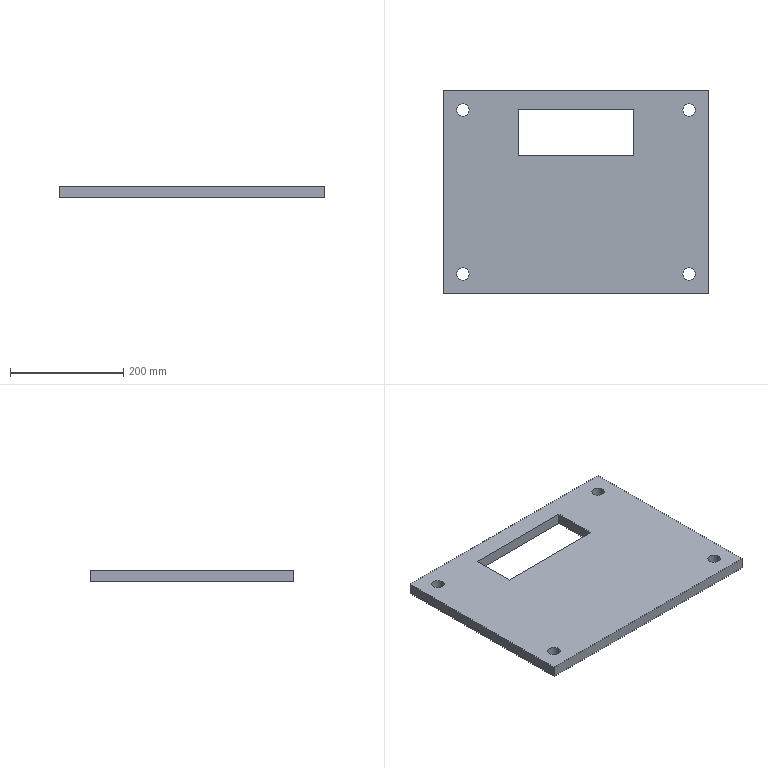Part | STEP file | Bearing seat fixing plate | 1 solid | 18 faces | box 470 x 360 x 20 mm | volume 3025589 mm3 | plane 10 | cylinder 8 | commonest cylinder face diameters 22 x8
STEP:
#1=CARTESIAN_POINT('',(0.,0.,0.));
#2=DIRECTION('',(0.,0.,1.));
#3=DIRECTION('',(1.,0.,0.));
#4=AXIS2_PLACEMENT_3D('',#1,#2,#3);
#5=CARTESIAN_POINT('',(424.,-325.,20.));
#6=VERTEX_POINT('',#5);
#7=CARTESIAN_POINT('',(424.,-325.,0.));
#8=VERTEX_POINT('',#7);
#9=CARTESIAN_POINT('',(424.,-325.,20.));
#10=DIRECTION('',(0.,0.,-1.));
#11=VECTOR('',#10,1.);
#12=LINE('',#9,#11);
#13=CARTESIAN_POINT('',(435.,-325.,20.));
#14=DIRECTION('',(0.,0.,-1.));
#15=DIRECTION('',(-1.,0.,0.));
#16=AXIS2_PLACEMENT_3D('',#13,#14,#15);
#17=CYLINDRICAL_SURFACE('',#16,11.);
#18=CARTESIAN_POINT('',(6.283,0.));
#19=DIRECTION('',(0.,1.));
#20=VECTOR('',#19,1.);
#21=LINE('',#18,#20);
#22=(GEOMETRIC_REPRESENTATION_CONTEXT(2)PARAMETRIC_REPRESENTATION_CONTEXT()REPRESENTATION_CONTEXT('',''));
#23=DEFINITIONAL_REPRESENTATION('',(#21),#22);
#24=PCURVE('',#17,#23);
#25=CARTESIAN_POINT('',(435.,-325.,20.));
#26=DIRECTION('',(0.,0.,-1.));
#27=DIRECTION('',(-1.,0.,0.));
#28=AXIS2_PLACEMENT_3D('',#25,#26,#27);
#29=CYLINDRICAL_SURFACE('',#28,11.);
#30=CARTESIAN_POINT('',(0.,0.));
#31=DIRECTION('',(0.,1.));
#32=VECTOR('',#31,1.);
#33=LINE('',#30,#32);
#34=(GEOMETRIC_REPRESENTATION_CONTEXT(2)PARAMETRIC_REPRESENTATION_CONTEXT()REPRESENTATION_CONTEXT('',''));
#35=DEFINITIONAL_REPRESENTATION('',(#33),#34);
#36=PCURVE('',#29,#35);
#37=SURFACE_CURVE('',#12,(#24,#36),.PCURVE_S1.);
#38=EDGE_CURVE('',#6,#8,#37,.T.);
#39=ORIENTED_EDGE('',*,*,#38,.T.);
#40=CARTESIAN_POINT('',(446.,-325.,0.));
#41=VERTEX_POINT('',#40);
#42=CARTESIAN_POINT('',(435.,-325.,0.));
#43=DIRECTION('',(0.,0.,1.));
#44=DIRECTION('',(1.,0.,0.));
#45=AXIS2_PLACEMENT_3D('',#42,#43,#44);
#46=CIRCLE('',#45,11.);
#47=CARTESIAN_POINT('',(9.425,20.));
#48=DIRECTION('',(-1.,0.));
#49=VECTOR('',#48,1.);
#50=LINE('',#47,#49);
#51=(GEOMETRIC_REPRESENTATION_CONTEXT(2)PARAMETRIC_REPRESENTATION_CONTEXT()REPRESENTATION_CONTEXT('',''));
#52=DEFINITIONAL_REPRESENTATION('',(#50),#51);
#53=PCURVE('',#17,#52);
#54=CARTESIAN_POINT('',(0.,0.,0.));
#55=DIRECTION('',(0.,0.,1.));
#56=DIRECTION('',(1.,0.,0.));
#57=AXIS2_PLACEMENT_3D('',#54,#55,#56);
#58=PLANE('',#57);
#59=CARTESIAN_POINT('',(435.,-325.));
#60=DIRECTION('',(1.,0.));
#61=AXIS2_PLACEMENT_2D('',#59,#60);
#62=CIRCLE('',#61,11.);
#63=(GEOMETRIC_REPRESENTATION_CONTEXT(2)PARAMETRIC_REPRESENTATION_CONTEXT()REPRESENTATION_CONTEXT('',''));
#64=DEFINITIONAL_REPRESENTATION('',(#62),#63);
#65=PCURVE('',#58,#64);
#66=SURFACE_CURVE('',#46,(#53,#65),.PCURVE_S1.);
#67=EDGE_CURVE('',#8,#41,#66,.T.);
#68=ORIENTED_EDGE('',*,*,#67,.T.);
#69=CARTESIAN_POINT('',(446.,-325.,20.));
#70=VERTEX_POINT('',#69);
#71=CARTESIAN_POINT('',(446.,-325.,20.));
#72=DIRECTION('',(0.,0.,-1.));
#73=VECTOR('',#72,1.);
#74=LINE('',#71,#73);
#75=CARTESIAN_POINT('',(3.142,0.));
#76=DIRECTION('',(0.,1.));
#77=VECTOR('',#76,1.);
#78=LINE('',#75,#77);
#79=(GEOMETRIC_REPRESENTATION_CONTEXT(2)PARAMETRIC_REPRESENTATION_CONTEXT()REPRESENTATION_CONTEXT('',''));
#80=DEFINITIONAL_REPRESENTATION('',(#78),#79);
#81=PCURVE('',#17,#80);
#82=CARTESIAN_POINT('',(3.142,0.));
#83=DIRECTION('',(0.,1.));
#84=VECTOR('',#83,1.);
#85=LINE('',#82,#84);
#86=(GEOMETRIC_REPRESENTATION_CONTEXT(2)PARAMETRIC_REPRESENTATION_CONTEXT()REPRESENTATION_CONTEXT('',''));
#87=DEFINITIONAL_REPRESENTATION('',(#85),#86);
#88=PCURVE('',#29,#87);
#89=SURFACE_CURVE('',#74,(#81,#88),.PCURVE_S1.);
#90=EDGE_CURVE('',#70,#41,#89,.T.);
#91=ORIENTED_EDGE('',*,*,#90,.F.);
#92=CARTESIAN_POINT('',(435.,-325.,20.));
#93=DIRECTION('',(0.,0.,1.));
#94=DIRECTION('',(1.,0.,0.));
#95=AXIS2_PLACEMENT_3D('',#92,#93,#94);
#96=CIRCLE('',#95,11.);
#97=CARTESIAN_POINT('',(9.425,0.));
#98=DIRECTION('',(-1.,0.));
#99=VECTOR('',#98,1.);
#100=LINE('',#97,#99);
#101=(GEOMETRIC_REPRESENTATION_CONTEXT(2)PARAMETRIC_REPRESENTATION_CONTEXT()REPRESENTATION_CONTEXT('',''));
#102=DEFINITIONAL_REPRESENTATION('',(#100),#101);
#103=PCURVE('',#17,#102);
#104=CARTESIAN_POINT('',(0.,0.,20.));
#105=DIRECTION('',(0.,0.,1.));
#106=DIRECTION('',(1.,0.,0.));
#107=AXIS2_PLACEMENT_3D('',#104,#105,#106);
#108=PLANE('',#107);
#109=CARTESIAN_POINT('',(435.,-325.));
#110=DIRECTION('',(1.,0.));
#111=AXIS2_PLACEMENT_2D('',#109,#110);
#112=CIRCLE('',#111,11.);
#113=(GEOMETRIC_REPRESENTATION_CONTEXT(2)PARAMETRIC_REPRESENTATION_CONTEXT()REPRESENTATION_CONTEXT('',''));
#114=DEFINITIONAL_REPRESENTATION('',(#112),#113);
#115=PCURVE('',#108,#114);
#116=SURFACE_CURVE('',#96,(#103,#115),.PCURVE_S1.);
#117=EDGE_CURVE('',#6,#70,#116,.T.);
#118=ORIENTED_EDGE('',*,*,#117,.F.);
#119=EDGE_LOOP('',(#39,#68,#91,#118));
#120=FACE_BOUND('',#119,.F.);
#121=ADVANCED_FACE('',(#120),#17,.F.);
#122=CARTESIAN_POINT('',(424.,-35.,20.));
#123=VERTEX_POINT('',#122);
#124=CARTESIAN_POINT('',(424.,-35.,0.));
#125=VERTEX_POINT('',#124);
#126=CARTESIAN_POINT('',(424.,-35.,20.));
#127=DIRECTION('',(0.,0.,-1.));
#128=VECTOR('',#127,1.);
#129=LINE('',#126,#128);
#130=CARTESIAN_POINT('',(435.,-35.,20.));
#131=DIRECTION('',(0.,0.,-1.));
#132=DIRECTION('',(-1.,0.,0.));
#133=AXIS2_PLACEMENT_3D('',#130,#131,#132);
#134=CYLINDRICAL_SURFACE('',#133,11.);
#135=CARTESIAN_POINT('',(6.283,0.));
#136=DIRECTION('',(0.,1.));
#137=VECTOR('',#136,1.);
#138=LINE('',#135,#137);
#139=(GEOMETRIC_REPRESENTATION_CONTEXT(2)PARAMETRIC_REPRESENTATION_CONTEXT()REPRESENTATION_CONTEXT('',''));
#140=DEFINITIONAL_REPRESENTATION('',(#138),#139);
#141=PCURVE('',#134,#140);
#142=CARTESIAN_POINT('',(435.,-35.,20.));
#143=DIRECTION('',(0.,0.,-1.));
#144=DIRECTION('',(-1.,0.,0.));
#145=AXIS2_PLACEMENT_3D('',#142,#143,#144);
#146=CYLINDRICAL_SURFACE('',#145,11.);
#147=CARTESIAN_POINT('',(0.,0.));
#148=DIRECTION('',(0.,1.));
#149=VECTOR('',#148,1.);
#150=LINE('',#147,#149);
#151=(GEOMETRIC_REPRESENTATION_CONTEXT(2)PARAMETRIC_REPRESENTATION_CONTEXT()REPRESENTATION_CONTEXT('',''));
#152=DEFINITIONAL_REPRESENTATION('',(#150),#151);
#153=PCURVE('',#146,#152);
#154=SURFACE_CURVE('',#129,(#141,#153),.PCURVE_S1.);
#155=EDGE_CURVE('',#123,#125,#154,.T.);
#156=ORIENTED_EDGE('',*,*,#155,.T.);
#157=CARTESIAN_POINT('',(446.,-35.,0.));
#158=VERTEX_POINT('',#157);
#159=CARTESIAN_POINT('',(435.,-35.,0.));
#160=DIRECTION('',(0.,0.,1.));
#161=DIRECTION('',(1.,0.,0.));
#162=AXIS2_PLACEMENT_3D('',#159,#160,#161);
#163=CIRCLE('',#162,11.);
#164=CARTESIAN_POINT('',(9.425,20.));
#165=DIRECTION('',(-1.,0.));
#166=VECTOR('',#165,1.);
#167=LINE('',#164,#166);
#168=(GEOMETRIC_REPRESENTATION_CONTEXT(2)PARAMETRIC_REPRESENTATION_CONTEXT()REPRESENTATION_CONTEXT('',''));
#169=DEFINITIONAL_REPRESENTATION('',(#167),#168);
#170=PCURVE('',#134,#169);
#171=CARTESIAN_POINT('',(435.,-35.));
#172=DIRECTION('',(1.,0.));
#173=AXIS2_PLACEMENT_2D('',#171,#172);
#174=CIRCLE('',#173,11.);
#175=(GEOMETRIC_REPRESENTATION_CONTEXT(2)PARAMETRIC_REPRESENTATION_CONTEXT()REPRESENTATION_CONTEXT('',''));
#176=DEFINITIONAL_REPRESENTATION('',(#174),#175);
#177=PCURVE('',#58,#176);
#178=SURFACE_CURVE('',#163,(#170,#177),.PCURVE_S1.);
#179=EDGE_CURVE('',#125,#158,#178,.T.);
#180=ORIENTED_EDGE('',*,*,#179,.T.);
#181=CARTESIAN_POINT('',(446.,-35.,20.));
#182=VERTEX_POINT('',#181);
#183=CARTESIAN_POINT('',(446.,-35.,20.));
#184=DIRECTION('',(0.,0.,-1.));
#185=VECTOR('',#184,1.);
#186=LINE('',#183,#185);
#187=CARTESIAN_POINT('',(3.142,0.));
#188=DIRECTION('',(0.,1.));
#189=VECTOR('',#188,1.);
#190=LINE('',#187,#189);
#191=(GEOMETRIC_REPRESENTATION_CONTEXT(2)PARAMETRIC_REPRESENTATION_CONTEXT()REPRESENTATION_CONTEXT('',''));
#192=DEFINITIONAL_REPRESENTATION('',(#190),#191);
#193=PCURVE('',#134,#192);
#194=CARTESIAN_POINT('',(3.142,0.));
#195=DIRECTION('',(0.,1.));
#196=VECTOR('',#195,1.);
#197=LINE('',#194,#196);
#198=(GEOMETRIC_REPRESENTATION_CONTEXT(2)PARAMETRIC_REPRESENTATION_CONTEXT()REPRESENTATION_CONTEXT('',''));
#199=DEFINITIONAL_REPRESENTATION('',(#197),#198);
#200=PCURVE('',#146,#199);
#201=SURFACE_CURVE('',#186,(#193,#200),.PCURVE_S1.);
#202=EDGE_CURVE('',#182,#158,#201,.T.);
#203=ORIENTED_EDGE('',*,*,#202,.F.);
#204=CARTESIAN_POINT('',(435.,-35.,20.));
#205=DIRECTION('',(0.,0.,1.));
#206=DIRECTION('',(1.,0.,0.));
#207=AXIS2_PLACEMENT_3D('',#204,#205,#206);
#208=CIRCLE('',#207,11.);
#209=CARTESIAN_POINT('',(9.425,0.));
#210=DIRECTION('',(-1.,0.));
#211=VECTOR('',#210,1.);
#212=LINE('',#209,#211);
#213=(GEOMETRIC_REPRESENTATION_CONTEXT(2)PARAMETRIC_REPRESENTATION_CONTEXT()REPRESENTATION_CONTEXT('',''));
#214=DEFINITIONAL_REPRESENTATION('',(#212),#213);
#215=PCURVE('',#134,#214);
#216=CARTESIAN_POINT('',(435.,-35.));
#217=DIRECTION('',(1.,0.));
#218=AXIS2_PLACEMENT_2D('',#216,#217);
#219=CIRCLE('',#218,11.);
#220=(GEOMETRIC_REPRESENTATION_CONTEXT(2)PARAMETRIC_REPRESENTATION_CONTEXT()REPRESENTATION_CONTEXT('',''));
#221=DEFINITIONAL_REPRESENTATION('',(#219),#220);
#222=PCURVE('',#108,#221);
#223=SURFACE_CURVE('',#208,(#215,#222),.PCURVE_S1.);
#224=EDGE_CURVE('',#123,#182,#223,.T.);
#225=ORIENTED_EDGE('',*,*,#224,.F.);
#226=EDGE_LOOP('',(#156,#180,#203,#225));
#227=FACE_BOUND('',#226,.F.);
#228=ADVANCED_FACE('',(#227),#134,.F.);
#229=CARTESIAN_POINT('',(24.,-325.,20.));
#230=VERTEX_POINT('',#229);
#231=CARTESIAN_POINT('',(24.,-325.,0.));
#232=VERTEX_POINT('',#231);
#233=CARTESIAN_POINT('',(24.,-325.,20.));
#234=DIRECTION('',(0.,0.,-1.));
#235=VECTOR('',#234,1.);
#236=LINE('',#233,#235);
#237=CARTESIAN_POINT('',(35.,-325.,20.));
#238=DIRECTION('',(0.,0.,-1.));
#239=DIRECTION('',(-1.,0.,0.));
#240=AXIS2_PLACEMENT_3D('',#237,#238,#239);
#241=CYLINDRICAL_SURFACE('',#240,11.);
#242=CARTESIAN_POINT('',(6.283,0.));
#243=DIRECTION('',(0.,1.));
#244=VECTOR('',#243,1.);
#245=LINE('',#242,#244);
#246=(GEOMETRIC_REPRESENTATION_CONTEXT(2)PARAMETRIC_REPRESENTATION_CONTEXT()REPRESENTATION_CONTEXT('',''));
#247=DEFINITIONAL_REPRESENTATION('',(#245),#246);
#248=PCURVE('',#241,#247);
#249=CARTESIAN_POINT('',(35.,-325.,20.));
#250=DIRECTION('',(0.,0.,-1.));
#251=DIRECTION('',(-1.,0.,0.));
#252=AXIS2_PLACEMENT_3D('',#249,#250,#251);
#253=CYLINDRICAL_SURFACE('',#252,11.);
#254=CARTESIAN_POINT('',(0.,0.));
#255=DIRECTION('',(0.,1.));
#256=VECTOR('',#255,1.);
#257=LINE('',#254,#256);
#258=(GEOMETRIC_REPRESENTATION_CONTEXT(2)PARAMETRIC_REPRESENTATION_CONTEXT()REPRESENTATION_CONTEXT('',''));
#259=DEFINITIONAL_REPRESENTATION('',(#257),#258);
#260=PCURVE('',#253,#259);
#261=SURFACE_CURVE('',#236,(#248,#260),.PCURVE_S1.);
#262=EDGE_CURVE('',#230,#232,#261,.T.);
#263=ORIENTED_EDGE('',*,*,#262,.T.);
#264=CARTESIAN_POINT('',(46.,-325.,0.));
#265=VERTEX_POINT('',#264);
#266=CARTESIAN_POINT('',(35.,-325.,0.));
#267=DIRECTION('',(0.,0.,1.));
#268=DIRECTION('',(1.,0.,0.));
#269=AXIS2_PLACEMENT_3D('',#266,#267,#268);
#270=CIRCLE('',#269,11.);
#271=CARTESIAN_POINT('',(9.425,20.));
#272=DIRECTION('',(-1.,0.));
#273=VECTOR('',#272,1.);
#274=LINE('',#271,#273);
#275=(GEOMETRIC_REPRESENTATION_CONTEXT(2)PARAMETRIC_REPRESENTATION_CONTEXT()REPRESENTATION_CONTEXT('',''));
#276=DEFINITIONAL_REPRESENTATION('',(#274),#275);
#277=PCURVE('',#241,#276);
#278=CARTESIAN_POINT('',(35.,-325.));
#279=DIRECTION('',(1.,0.));
#280=AXIS2_PLACEMENT_2D('',#278,#279);
#281=CIRCLE('',#280,11.);
#282=(GEOMETRIC_REPRESENTATION_CONTEXT(2)PARAMETRIC_REPRESENTATION_CONTEXT()REPRESENTATION_CONTEXT('',''));
#283=DEFINITIONAL_REPRESENTATION('',(#281),#282);
#284=PCURVE('',#58,#283);
#285=SURFACE_CURVE('',#270,(#277,#284),.PCURVE_S1.);
#286=EDGE_CURVE('',#232,#265,#285,.T.);
#287=ORIENTED_EDGE('',*,*,#286,.T.);
#288=CARTESIAN_POINT('',(46.,-325.,20.));
#289=VERTEX_POINT('',#288);
#290=CARTESIAN_POINT('',(46.,-325.,20.));
#291=DIRECTION('',(0.,0.,-1.));
#292=VECTOR('',#291,1.);
#293=LINE('',#290,#292);
#294=CARTESIAN_POINT('',(3.142,0.));
#295=DIRECTION('',(0.,1.));
#296=VECTOR('',#295,1.);
#297=LINE('',#294,#296);
#298=(GEOMETRIC_REPRESENTATION_CONTEXT(2)PARAMETRIC_REPRESENTATION_CONTEXT()REPRESENTATION_CONTEXT('',''));
#299=DEFINITIONAL_REPRESENTATION('',(#297),#298);
#300=PCURVE('',#241,#299);
#301=CARTESIAN_POINT('',(3.142,0.));
#302=DIRECTION('',(0.,1.));
#303=VECTOR('',#302,1.);
#304=LINE('',#301,#303);
#305=(GEOMETRIC_REPRESENTATION_CONTEXT(2)PARAMETRIC_REPRESENTATION_CONTEXT()REPRESENTATION_CONTEXT('',''));
#306=DEFINITIONAL_REPRESENTATION('',(#304),#305);
#307=PCURVE('',#253,#306);
#308=SURFACE_CURVE('',#293,(#300,#307),.PCURVE_S1.);
#309=EDGE_CURVE('',#289,#265,#308,.T.);
#310=ORIENTED_EDGE('',*,*,#309,.F.);
#311=CARTESIAN_POINT('',(35.,-325.,20.));
#312=DIRECTION('',(0.,0.,1.));
#313=DIRECTION('',(1.,0.,0.));
#314=AXIS2_PLACEMENT_3D('',#311,#312,#313);
#315=CIRCLE('',#314,11.);
#316=CARTESIAN_POINT('',(9.425,0.));
#317=DIRECTION('',(-1.,0.));
#318=VECTOR('',#317,1.);
#319=LINE('',#316,#318);
#320=(GEOMETRIC_REPRESENTATION_CONTEXT(2)PARAMETRIC_REPRESENTATION_CONTEXT()REPRESENTATION_CONTEXT('',''));
#321=DEFINITIONAL_REPRESENTATION('',(#319),#320);
#322=PCURVE('',#241,#321);
#323=CARTESIAN_POINT('',(35.,-325.));
#324=DIRECTION('',(1.,0.));
#325=AXIS2_PLACEMENT_2D('',#323,#324);
#326=CIRCLE('',#325,11.);
#327=(GEOMETRIC_REPRESENTATION_CONTEXT(2)PARAMETRIC_REPRESENTATION_CONTEXT()REPRESENTATION_CONTEXT('',''));
#328=DEFINITIONAL_REPRESENTATION('',(#326),#327);
#329=PCURVE('',#108,#328);
#330=SURFACE_CURVE('',#315,(#322,#329),.PCURVE_S1.);
#331=EDGE_CURVE('',#230,#289,#330,.T.);
#332=ORIENTED_EDGE('',*,*,#331,.F.);
#333=EDGE_LOOP('',(#263,#287,#310,#332));
#334=FACE_BOUND('',#333,.F.);
#335=ADVANCED_FACE('',(#334),#241,.F.);
#336=CARTESIAN_POINT('',(24.,-35.,20.));
#337=VERTEX_POINT('',#336);
#338=CARTESIAN_POINT('',(24.,-35.,0.));
#339=VERTEX_POINT('',#338);
#340=CARTESIAN_POINT('',(24.,-35.,20.));
#341=DIRECTION('',(0.,0.,-1.));
#342=VECTOR('',#341,1.);
#343=LINE('',#340,#342);
#344=CARTESIAN_POINT('',(35.,-35.,20.));
#345=DIRECTION('',(0.,0.,-1.));
#346=DIRECTION('',(-1.,0.,0.));
#347=AXIS2_PLACEMENT_3D('',#344,#345,#346);
#348=CYLINDRICAL_SURFACE('',#347,11.);
#349=CARTESIAN_POINT('',(6.283,0.));
#350=DIRECTION('',(0.,1.));
#351=VECTOR('',#350,1.);
#352=LINE('',#349,#351);
#353=(GEOMETRIC_REPRESENTATION_CONTEXT(2)PARAMETRIC_REPRESENTATION_CONTEXT()REPRESENTATION_CONTEXT('',''));
#354=DEFINITIONAL_REPRESENTATION('',(#352),#353);
#355=PCURVE('',#348,#354);
#356=CARTESIAN_POINT('',(35.,-35.,20.));
#357=DIRECTION('',(0.,0.,-1.));
#358=DIRECTION('',(-1.,0.,0.));
#359=AXIS2_PLACEMENT_3D('',#356,#357,#358);
#360=CYLINDRICAL_SURFACE('',#359,11.);
#361=CARTESIAN_POINT('',(0.,0.));
#362=DIRECTION('',(0.,1.));
#363=VECTOR('',#362,1.);
#364=LINE('',#361,#363);
#365=(GEOMETRIC_REPRESENTATION_CONTEXT(2)PARAMETRIC_REPRESENTATION_CONTEXT()REPRESENTATION_CONTEXT('',''));
#366=DEFINITIONAL_REPRESENTATION('',(#364),#365);
#367=PCURVE('',#360,#366);
#368=SURFACE_CURVE('',#343,(#355,#367),.PCURVE_S1.);
#369=EDGE_CURVE('',#337,#339,#368,.T.);
#370=ORIENTED_EDGE('',*,*,#369,.T.);
#371=CARTESIAN_POINT('',(46.,-35.,0.));
#372=VERTEX_POINT('',#371);
#373=CARTESIAN_POINT('',(35.,-35.,0.));
#374=DIRECTION('',(0.,0.,1.));
#375=DIRECTION('',(1.,0.,0.));
#376=AXIS2_PLACEMENT_3D('',#373,#374,#375);
#377=CIRCLE('',#376,11.);
#378=CARTESIAN_POINT('',(9.425,20.));
#379=DIRECTION('',(-1.,0.));
#380=VECTOR('',#379,1.);
#381=LINE('',#378,#380);
#382=(GEOMETRIC_REPRESENTATION_CONTEXT(2)PARAMETRIC_REPRESENTATION_CONTEXT()REPRESENTATION_CONTEXT('',''));
#383=DEFINITIONAL_REPRESENTATION('',(#381),#382);
#384=PCURVE('',#348,#383);
#385=CARTESIAN_POINT('',(35.,-35.));
#386=DIRECTION('',(1.,0.));
#387=AXIS2_PLACEMENT_2D('',#385,#386);
#388=CIRCLE('',#387,11.);
#389=(GEOMETRIC_REPRESENTATION_CONTEXT(2)PARAMETRIC_REPRESENTATION_CONTEXT()REPRESENTATION_CONTEXT('',''));
#390=DEFINITIONAL_REPRESENTATION('',(#388),#389);
#391=PCURVE('',#58,#390);
#392=SURFACE_CURVE('',#377,(#384,#391),.PCURVE_S1.);
#393=EDGE_CURVE('',#339,#372,#392,.T.);
#394=ORIENTED_EDGE('',*,*,#393,.T.);
#395=CARTESIAN_POINT('',(46.,-35.,20.));
#396=VERTEX_POINT('',#395);
#397=CARTESIAN_POINT('',(46.,-35.,20.));
#398=DIRECTION('',(0.,0.,-1.));
#399=VECTOR('',#398,1.);
#400=LINE('',#397,#399);
#401=CARTESIAN_POINT('',(3.142,0.));
#402=DIRECTION('',(0.,1.));
#403=VECTOR('',#402,1.);
#404=LINE('',#401,#403);
#405=(GEOMETRIC_REPRESENTATION_CONTEXT(2)PARAMETRIC_REPRESENTATION_CONTEXT()REPRESENTATION_CONTEXT('',''));
#406=DEFINITIONAL_REPRESENTATION('',(#404),#405);
#407=PCURVE('',#348,#406);
#408=CARTESIAN_POINT('',(3.142,0.));
#409=DIRECTION('',(0.,1.));
#410=VECTOR('',#409,1.);
#411=LINE('',#408,#410);
#412=(GEOMETRIC_REPRESENTATION_CONTEXT(2)PARAMETRIC_REPRESENTATION_CONTEXT()REPRESENTATION_CONTEXT('',''));
#413=DEFINITIONAL_REPRESENTATION('',(#411),#412);
#414=PCURVE('',#360,#413);
#415=SURFACE_CURVE('',#400,(#407,#414),.PCURVE_S1.);
#416=EDGE_CURVE('',#396,#372,#415,.T.);
#417=ORIENTED_EDGE('',*,*,#416,.F.);
#418=CARTESIAN_POINT('',(35.,-35.,20.));
#419=DIRECTION('',(0.,0.,1.));
#420=DIRECTION('',(1.,0.,0.));
#421=AXIS2_PLACEMENT_3D('',#418,#419,#420);
#422=CIRCLE('',#421,11.);
#423=CARTESIAN_POINT('',(9.425,0.));
#424=DIRECTION('',(-1.,0.));
#425=VECTOR('',#424,1.);
#426=LINE('',#423,#425);
#427=(GEOMETRIC_REPRESENTATION_CONTEXT(2)PARAMETRIC_REPRESENTATION_CONTEXT()REPRESENTATION_CONTEXT('',''));
#428=DEFINITIONAL_REPRESENTATION('',(#426),#427);
#429=PCURVE('',#348,#428);
#430=CARTESIAN_POINT('',(35.,-35.));
#431=DIRECTION('',(1.,0.));
#432=AXIS2_PLACEMENT_2D('',#430,#431);
#433=CIRCLE('',#432,11.);
#434=(GEOMETRIC_REPRESENTATION_CONTEXT(2)PARAMETRIC_REPRESENTATION_CONTEXT()REPRESENTATION_CONTEXT('',''));
#435=DEFINITIONAL_REPRESENTATION('',(#433),#434);
#436=PCURVE('',#108,#435);
#437=SURFACE_CURVE('',#422,(#429,#436),.PCURVE_S1.);
#438=EDGE_CURVE('',#337,#396,#437,.T.);
#439=ORIENTED_EDGE('',*,*,#438,.F.);
#440=EDGE_LOOP('',(#370,#394,#417,#439));
#441=FACE_BOUND('',#440,.F.);
#442=ADVANCED_FACE('',(#441),#348,.F.);
#443=ORIENTED_EDGE('',*,*,#224,.F.);
#444=CARTESIAN_POINT('',(435.,-35.,20.));
#445=DIRECTION('',(0.,0.,1.));
#446=DIRECTION('',(1.,0.,0.));
#447=AXIS2_PLACEMENT_3D('',#444,#445,#446);
#448=CIRCLE('',#447,11.);
#449=CARTESIAN_POINT('',(435.,-35.));
#450=DIRECTION('',(1.,0.));
#451=AXIS2_PLACEMENT_2D('',#449,#450);
#452=CIRCLE('',#451,11.);
#453=(GEOMETRIC_REPRESENTATION_CONTEXT(2)PARAMETRIC_REPRESENTATION_CONTEXT()REPRESENTATION_CONTEXT('',''));
#454=DEFINITIONAL_REPRESENTATION('',(#452),#453);
#455=PCURVE('',#108,#454);
#456=CARTESIAN_POINT('',(3.142,0.));
#457=DIRECTION('',(-1.,0.));
#458=VECTOR('',#457,1.);
#459=LINE('',#456,#458);
#460=(GEOMETRIC_REPRESENTATION_CONTEXT(2)PARAMETRIC_REPRESENTATION_CONTEXT()REPRESENTATION_CONTEXT('',''));
#461=DEFINITIONAL_REPRESENTATION('',(#459),#460);
#462=PCURVE('',#146,#461);
#463=SURFACE_CURVE('',#448,(#455,#462),.PCURVE_S1.);
#464=EDGE_CURVE('',#182,#123,#463,.T.);
#465=ORIENTED_EDGE('',*,*,#464,.F.);
#466=EDGE_LOOP('',(#443,#465));
#467=FACE_BOUND('',#466,.T.);
#468=ORIENTED_EDGE('',*,*,#438,.F.);
#469=CARTESIAN_POINT('',(35.,-35.,20.));
#470=DIRECTION('',(0.,0.,1.));
#471=DIRECTION('',(1.,0.,0.));
#472=AXIS2_PLACEMENT_3D('',#469,#470,#471);
#473=CIRCLE('',#472,11.);
#474=CARTESIAN_POINT('',(35.,-35.));
#475=DIRECTION('',(1.,0.));
#476=AXIS2_PLACEMENT_2D('',#474,#475);
#477=CIRCLE('',#476,11.);
#478=(GEOMETRIC_REPRESENTATION_CONTEXT(2)PARAMETRIC_REPRESENTATION_CONTEXT()REPRESENTATION_CONTEXT('',''));
#479=DEFINITIONAL_REPRESENTATION('',(#477),#478);
#480=PCURVE('',#108,#479);
#481=CARTESIAN_POINT('',(3.142,0.));
#482=DIRECTION('',(-1.,0.));
#483=VECTOR('',#482,1.);
#484=LINE('',#481,#483);
#485=(GEOMETRIC_REPRESENTATION_CONTEXT(2)PARAMETRIC_REPRESENTATION_CONTEXT()REPRESENTATION_CONTEXT('',''));
#486=DEFINITIONAL_REPRESENTATION('',(#484),#485);
#487=PCURVE('',#360,#486);
#488=SURFACE_CURVE('',#473,(#480,#487),.PCURVE_S1.);
#489=EDGE_CURVE('',#396,#337,#488,.T.);
#490=ORIENTED_EDGE('',*,*,#489,.F.);
#491=EDGE_LOOP('',(#468,#490));
#492=FACE_BOUND('',#491,.T.);
#493=CARTESIAN_POINT('',(0.,0.,20.));
#494=VERTEX_POINT('',#493);
#495=CARTESIAN_POINT('',(0.,-360.,20.));
#496=VERTEX_POINT('',#495);
#497=CARTESIAN_POINT('',(0.,0.,20.));
#498=DIRECTION('',(0.,-1.,0.));
#499=VECTOR('',#498,1.);
#500=LINE('',#497,#499);
#501=CARTESIAN_POINT('',(0.,0.));
#502=DIRECTION('',(0.,-1.));
#503=VECTOR('',#502,1.);
#504=LINE('',#501,#503);
#505=(GEOMETRIC_REPRESENTATION_CONTEXT(2)PARAMETRIC_REPRESENTATION_CONTEXT()REPRESENTATION_CONTEXT('',''));
#506=DEFINITIONAL_REPRESENTATION('',(#504),#505);
#507=PCURVE('',#108,#506);
#508=CARTESIAN_POINT('',(0.,0.,20.));
#509=DIRECTION('',(1.,0.,0.));
#510=DIRECTION('',(0.,1.,0.));
#511=AXIS2_PLACEMENT_3D('',#508,#509,#510);
#512=PLANE('',#511);
#513=CARTESIAN_POINT('',(0.,0.));
#514=DIRECTION('',(-1.,0.));
#515=VECTOR('',#514,1.);
#516=LINE('',#513,#515);
#517=(GEOMETRIC_REPRESENTATION_CONTEXT(2)PARAMETRIC_REPRESENTATION_CONTEXT()REPRESENTATION_CONTEXT('',''));
#518=DEFINITIONAL_REPRESENTATION('',(#516),#517);
#519=PCURVE('',#512,#518);
#520=SURFACE_CURVE('',#500,(#507,#519),.PCURVE_S1.);
#521=EDGE_CURVE('',#494,#496,#520,.T.);
#522=ORIENTED_EDGE('',*,*,#521,.T.);
#523=CARTESIAN_POINT('',(470.,-360.,20.));
#524=VERTEX_POINT('',#523);
#525=CARTESIAN_POINT('',(0.,-360.,20.));
#526=DIRECTION('',(1.,0.,0.));
#527=VECTOR('',#526,1.);
#528=LINE('',#525,#527);
#529=CARTESIAN_POINT('',(0.,-360.));
#530=DIRECTION('',(1.,0.));
#531=VECTOR('',#530,1.);
#532=LINE('',#529,#531);
#533=(GEOMETRIC_REPRESENTATION_CONTEXT(2)PARAMETRIC_REPRESENTATION_CONTEXT()REPRESENTATION_CONTEXT('',''));
#534=DEFINITIONAL_REPRESENTATION('',(#532),#533);
#535=PCURVE('',#108,#534);
#536=CARTESIAN_POINT('',(0.,-360.,20.));
#537=DIRECTION('',(0.,1.,0.));
#538=DIRECTION('',(0.,0.,1.));
#539=AXIS2_PLACEMENT_3D('',#536,#537,#538);
#540=PLANE('',#539);
#541=CARTESIAN_POINT('',(0.,0.));
#542=DIRECTION('',(0.,1.));
#543=VECTOR('',#542,1.);
#544=LINE('',#541,#543);
#545=(GEOMETRIC_REPRESENTATION_CONTEXT(2)PARAMETRIC_REPRESENTATION_CONTEXT()REPRESENTATION_CONTEXT('',''));
#546=DEFINITIONAL_REPRESENTATION('',(#544),#545);
#547=PCURVE('',#540,#546);
#548=SURFACE_CURVE('',#528,(#535,#547),.PCURVE_S1.);
#549=EDGE_CURVE('',#496,#524,#548,.T.);
#550=ORIENTED_EDGE('',*,*,#549,.T.);
#551=CARTESIAN_POINT('',(470.,0.,20.));
#552=VERTEX_POINT('',#551);
#553=CARTESIAN_POINT('',(470.,0.,20.));
#554=DIRECTION('',(0.,1.,0.));
#555=VECTOR('',#554,1.);
#556=LINE('',#553,#555);
#557=CARTESIAN_POINT('',(470.,0.));
#558=DIRECTION('',(0.,1.));
#559=VECTOR('',#558,1.);
#560=LINE('',#557,#559);
#561=(GEOMETRIC_REPRESENTATION_CONTEXT(2)PARAMETRIC_REPRESENTATION_CONTEXT()REPRESENTATION_CONTEXT('',''));
#562=DEFINITIONAL_REPRESENTATION('',(#560),#561);
#563=PCURVE('',#108,#562);
#564=CARTESIAN_POINT('',(470.,0.,20.));
#565=DIRECTION('',(-1.,0.,0.));
#566=DIRECTION('',(0.,-1.,0.));
#567=AXIS2_PLACEMENT_3D('',#564,#565,#566);
#568=PLANE('',#567);
#569=CARTESIAN_POINT('',(0.,0.));
#570=DIRECTION('',(-1.,0.));
#571=VECTOR('',#570,1.);
#572=LINE('',#569,#571);
#573=(GEOMETRIC_REPRESENTATION_CONTEXT(2)PARAMETRIC_REPRESENTATION_CONTEXT()REPRESENTATION_CONTEXT('',''));
#574=DEFINITIONAL_REPRESENTATION('',(#572),#573);
#575=PCURVE('',#568,#574);
#576=SURFACE_CURVE('',#556,(#563,#575),.PCURVE_S1.);
#577=EDGE_CURVE('',#524,#552,#576,.T.);
#578=ORIENTED_EDGE('',*,*,#577,.T.);
#579=CARTESIAN_POINT('',(0.,0.,20.));
#580=DIRECTION('',(-1.,0.,0.));
#581=VECTOR('',#580,1.);
#582=LINE('',#579,#581);
#583=CARTESIAN_POINT('',(0.,0.));
#584=DIRECTION('',(-1.,0.));
#585=VECTOR('',#584,1.);
#586=LINE('',#583,#585);
#587=(GEOMETRIC_REPRESENTATION_CONTEXT(2)PARAMETRIC_REPRESENTATION_CONTEXT()REPRESENTATION_CONTEXT('',''));
#588=DEFINITIONAL_REPRESENTATION('',(#586),#587);
#589=PCURVE('',#108,#588);
#590=CARTESIAN_POINT('',(0.,0.,20.));
#591=DIRECTION('',(0.,-1.,0.));
#592=DIRECTION('',(0.,0.,-1.));
#593=AXIS2_PLACEMENT_3D('',#590,#591,#592);
#594=PLANE('',#593);
#595=CARTESIAN_POINT('',(0.,0.));
#596=DIRECTION('',(0.,-1.));
#597=VECTOR('',#596,1.);
#598=LINE('',#595,#597);
#599=(GEOMETRIC_REPRESENTATION_CONTEXT(2)PARAMETRIC_REPRESENTATION_CONTEXT()REPRESENTATION_CONTEXT('',''));
#600=DEFINITIONAL_REPRESENTATION('',(#598),#599);
#601=PCURVE('',#594,#600);
#602=SURFACE_CURVE('',#582,(#589,#601),.PCURVE_S1.);
#603=EDGE_CURVE('',#552,#494,#602,.T.);
#604=ORIENTED_EDGE('',*,*,#603,.T.);
#605=EDGE_LOOP('',(#522,#550,#578,#604));
#606=FACE_BOUND('',#605,.T.);
#607=CARTESIAN_POINT('',(132.5,-115.,20.));
#608=VERTEX_POINT('',#607);
#609=CARTESIAN_POINT('',(337.5,-115.,20.));
#610=VERTEX_POINT('',#609);
#611=CARTESIAN_POINT('',(132.5,-115.,20.));
#612=DIRECTION('',(1.,0.,0.));
#613=VECTOR('',#612,1.);
#614=LINE('',#611,#613);
#615=CARTESIAN_POINT('',(132.5,-115.));
#616=DIRECTION('',(1.,0.));
#617=VECTOR('',#616,1.);
#618=LINE('',#615,#617);
#619=(GEOMETRIC_REPRESENTATION_CONTEXT(2)PARAMETRIC_REPRESENTATION_CONTEXT()REPRESENTATION_CONTEXT('',''));
#620=DEFINITIONAL_REPRESENTATION('',(#618),#619);
#621=PCURVE('',#108,#620);
#622=CARTESIAN_POINT('',(132.5,-115.,20.));
#623=DIRECTION('',(0.,1.,0.));
#624=DIRECTION('',(-1.,0.,0.));
#625=AXIS2_PLACEMENT_3D('',#622,#623,#624);
#626=PLANE('',#625);
#627=CARTESIAN_POINT('',(0.,0.));
#628=DIRECTION('',(-1.,0.));
#629=VECTOR('',#628,1.);
#630=LINE('',#627,#629);
#631=(GEOMETRIC_REPRESENTATION_CONTEXT(2)PARAMETRIC_REPRESENTATION_CONTEXT()REPRESENTATION_CONTEXT('',''));
#632=DEFINITIONAL_REPRESENTATION('',(#630),#631);
#633=PCURVE('',#626,#632);
#634=SURFACE_CURVE('',#614,(#621,#633),.PCURVE_S1.);
#635=EDGE_CURVE('',#608,#610,#634,.T.);
#636=ORIENTED_EDGE('',*,*,#635,.F.);
#637=CARTESIAN_POINT('',(132.5,-35.,20.));
#638=VERTEX_POINT('',#637);
#639=CARTESIAN_POINT('',(132.5,-35.,20.));
#640=DIRECTION('',(0.,-1.,0.));
#641=VECTOR('',#640,1.);
#642=LINE('',#639,#641);
#643=CARTESIAN_POINT('',(132.5,-35.));
#644=DIRECTION('',(0.,-1.));
#645=VECTOR('',#644,1.);
#646=LINE('',#643,#645);
#647=(GEOMETRIC_REPRESENTATION_CONTEXT(2)PARAMETRIC_REPRESENTATION_CONTEXT()REPRESENTATION_CONTEXT('',''));
#648=DEFINITIONAL_REPRESENTATION('',(#646),#647);
#649=PCURVE('',#108,#648);
#650=CARTESIAN_POINT('',(132.5,-35.,20.));
#651=DIRECTION('',(1.,0.,0.));
#652=DIRECTION('',(0.,1.,0.));
#653=AXIS2_PLACEMENT_3D('',#650,#651,#652);
#654=PLANE('',#653);
#655=CARTESIAN_POINT('',(0.,0.));
#656=DIRECTION('',(-1.,0.));
#657=VECTOR('',#656,1.);
#658=LINE('',#655,#657);
#659=(GEOMETRIC_REPRESENTATION_CONTEXT(2)PARAMETRIC_REPRESENTATION_CONTEXT()REPRESENTATION_CONTEXT('',''));
#660=DEFINITIONAL_REPRESENTATION('',(#658),#659);
#661=PCURVE('',#654,#660);
#662=SURFACE_CURVE('',#642,(#649,#661),.PCURVE_S1.);
#663=EDGE_CURVE('',#638,#608,#662,.T.);
#664=ORIENTED_EDGE('',*,*,#663,.F.);
#665=CARTESIAN_POINT('',(337.5,-35.,20.));
#666=VERTEX_POINT('',#665);
#667=CARTESIAN_POINT('',(132.5,-35.,20.));
#668=DIRECTION('',(-1.,0.,0.));
#669=VECTOR('',#668,1.);
#670=LINE('',#667,#669);
#671=CARTESIAN_POINT('',(132.5,-35.));
#672=DIRECTION('',(-1.,0.));
#673=VECTOR('',#672,1.);
#674=LINE('',#671,#673);
#675=(GEOMETRIC_REPRESENTATION_CONTEXT(2)PARAMETRIC_REPRESENTATION_CONTEXT()REPRESENTATION_CONTEXT('',''));
#676=DEFINITIONAL_REPRESENTATION('',(#674),#675);
#677=PCURVE('',#108,#676);
#678=CARTESIAN_POINT('',(132.5,-35.,20.));
#679=DIRECTION('',(0.,-1.,0.));
#680=DIRECTION('',(1.,0.,0.));
#681=AXIS2_PLACEMENT_3D('',#678,#679,#680);
#682=PLANE('',#681);
#683=CARTESIAN_POINT('',(0.,0.));
#684=DIRECTION('',(-1.,0.));
#685=VECTOR('',#684,1.);
#686=LINE('',#683,#685);
#687=(GEOMETRIC_REPRESENTATION_CONTEXT(2)PARAMETRIC_REPRESENTATION_CONTEXT()REPRESENTATION_CONTEXT('',''));
#688=DEFINITIONAL_REPRESENTATION('',(#686),#687);
#689=PCURVE('',#682,#688);
#690=SURFACE_CURVE('',#670,(#677,#689),.PCURVE_S1.);
#691=EDGE_CURVE('',#666,#638,#690,.T.);
#692=ORIENTED_EDGE('',*,*,#691,.F.);
#693=CARTESIAN_POINT('',(337.5,-35.,20.));
#694=DIRECTION('',(0.,1.,0.));
#695=VECTOR('',#694,1.);
#696=LINE('',#693,#695);
#697=CARTESIAN_POINT('',(337.5,-35.));
#698=DIRECTION('',(0.,1.));
#699=VECTOR('',#698,1.);
#700=LINE('',#697,#699);
#701=(GEOMETRIC_REPRESENTATION_CONTEXT(2)PARAMETRIC_REPRESENTATION_CONTEXT()REPRESENTATION_CONTEXT('',''));
#702=DEFINITIONAL_REPRESENTATION('',(#700),#701);
#703=PCURVE('',#108,#702);
#704=CARTESIAN_POINT('',(337.5,-35.,20.));
#705=DIRECTION('',(-1.,0.,0.));
#706=DIRECTION('',(0.,-1.,0.));
#707=AXIS2_PLACEMENT_3D('',#704,#705,#706);
#708=PLANE('',#707);
#709=CARTESIAN_POINT('',(0.,0.));
#710=DIRECTION('',(-1.,0.));
#711=VECTOR('',#710,1.);
#712=LINE('',#709,#711);
#713=(GEOMETRIC_REPRESENTATION_CONTEXT(2)PARAMETRIC_REPRESENTATION_CONTEXT()REPRESENTATION_CONTEXT('',''));
#714=DEFINITIONAL_REPRESENTATION('',(#712),#713);
#715=PCURVE('',#708,#714);
#716=SURFACE_CURVE('',#696,(#703,#715),.PCURVE_S1.);
#717=EDGE_CURVE('',#610,#666,#716,.T.);
#718=ORIENTED_EDGE('',*,*,#717,.F.);
#719=EDGE_LOOP('',(#636,#664,#692,#718));
#720=FACE_BOUND('',#719,.T.);
#721=ORIENTED_EDGE('',*,*,#331,.F.);
#722=CARTESIAN_POINT('',(35.,-325.,20.));
#723=DIRECTION('',(0.,0.,1.));
#724=DIRECTION('',(1.,0.,0.));
#725=AXIS2_PLACEMENT_3D('',#722,#723,#724);
#726=CIRCLE('',#725,11.);
#727=CARTESIAN_POINT('',(35.,-325.));
#728=DIRECTION('',(1.,0.));
#729=AXIS2_PLACEMENT_2D('',#727,#728);
#730=CIRCLE('',#729,11.);
#731=(GEOMETRIC_REPRESENTATION_CONTEXT(2)PARAMETRIC_REPRESENTATION_CONTEXT()REPRESENTATION_CONTEXT('',''));
#732=DEFINITIONAL_REPRESENTATION('',(#730),#731);
#733=PCURVE('',#108,#732);
#734=CARTESIAN_POINT('',(3.142,0.));
#735=DIRECTION('',(-1.,0.));
#736=VECTOR('',#735,1.);
#737=LINE('',#734,#736);
#738=(GEOMETRIC_REPRESENTATION_CONTEXT(2)PARAMETRIC_REPRESENTATION_CONTEXT()REPRESENTATION_CONTEXT('',''));
#739=DEFINITIONAL_REPRESENTATION('',(#737),#738);
#740=PCURVE('',#253,#739);
#741=SURFACE_CURVE('',#726,(#733,#740),.PCURVE_S1.);
#742=EDGE_CURVE('',#289,#230,#741,.T.);
#743=ORIENTED_EDGE('',*,*,#742,.F.);
#744=EDGE_LOOP('',(#721,#743));
#745=FACE_BOUND('',#744,.T.);
#746=ORIENTED_EDGE('',*,*,#117,.F.);
#747=CARTESIAN_POINT('',(435.,-325.,20.));
#748=DIRECTION('',(0.,0.,1.));
#749=DIRECTION('',(1.,0.,0.));
#750=AXIS2_PLACEMENT_3D('',#747,#748,#749);
#751=CIRCLE('',#750,11.);
#752=CARTESIAN_POINT('',(435.,-325.));
#753=DIRECTION('',(1.,0.));
#754=AXIS2_PLACEMENT_2D('',#752,#753);
#755=CIRCLE('',#754,11.);
#756=(GEOMETRIC_REPRESENTATION_CONTEXT(2)PARAMETRIC_REPRESENTATION_CONTEXT()REPRESENTATION_CONTEXT('',''));
#757=DEFINITIONAL_REPRESENTATION('',(#755),#756);
#758=PCURVE('',#108,#757);
#759=CARTESIAN_POINT('',(3.142,0.));
#760=DIRECTION('',(-1.,0.));
#761=VECTOR('',#760,1.);
#762=LINE('',#759,#761);
#763=(GEOMETRIC_REPRESENTATION_CONTEXT(2)PARAMETRIC_REPRESENTATION_CONTEXT()REPRESENTATION_CONTEXT('',''));
#764=DEFINITIONAL_REPRESENTATION('',(#762),#763);
#765=PCURVE('',#29,#764);
#766=SURFACE_CURVE('',#751,(#758,#765),.PCURVE_S1.);
#767=EDGE_CURVE('',#70,#6,#766,.T.);
#768=ORIENTED_EDGE('',*,*,#767,.F.);
#769=EDGE_LOOP('',(#746,#768));
#770=FACE_BOUND('',#769,.T.);
#771=ADVANCED_FACE('',(#467,#492,#606,#720,#745,#770),#108,.T.);
#772=ORIENTED_EDGE('',*,*,#179,.T.);
#773=CARTESIAN_POINT('',(435.,-35.,0.));
#774=DIRECTION('',(0.,0.,1.));
#775=DIRECTION('',(1.,0.,0.));
#776=AXIS2_PLACEMENT_3D('',#773,#774,#775);
#777=CIRCLE('',#776,11.);
#778=CARTESIAN_POINT('',(435.,-35.));
#779=DIRECTION('',(1.,0.));
#780=AXIS2_PLACEMENT_2D('',#778,#779);
#781=CIRCLE('',#780,11.);
#782=(GEOMETRIC_REPRESENTATION_CONTEXT(2)PARAMETRIC_REPRESENTATION_CONTEXT()REPRESENTATION_CONTEXT('',''));
#783=DEFINITIONAL_REPRESENTATION('',(#781),#782);
#784=PCURVE('',#58,#783);
#785=CARTESIAN_POINT('',(3.142,20.));
#786=DIRECTION('',(-1.,0.));
#787=VECTOR('',#786,1.);
#788=LINE('',#785,#787);
#789=(GEOMETRIC_REPRESENTATION_CONTEXT(2)PARAMETRIC_REPRESENTATION_CONTEXT()REPRESENTATION_CONTEXT('',''));
#790=DEFINITIONAL_REPRESENTATION('',(#788),#789);
#791=PCURVE('',#146,#790);
#792=SURFACE_CURVE('',#777,(#784,#791),.PCURVE_S1.);
#793=EDGE_CURVE('',#158,#125,#792,.T.);
#794=ORIENTED_EDGE('',*,*,#793,.T.);
#795=EDGE_LOOP('',(#772,#794));
#796=FACE_BOUND('',#795,.T.);
#797=ORIENTED_EDGE('',*,*,#393,.T.);
#798=CARTESIAN_POINT('',(35.,-35.,0.));
#799=DIRECTION('',(0.,0.,1.));
#800=DIRECTION('',(1.,0.,0.));
#801=AXIS2_PLACEMENT_3D('',#798,#799,#800);
#802=CIRCLE('',#801,11.);
#803=CARTESIAN_POINT('',(35.,-35.));
#804=DIRECTION('',(1.,0.));
#805=AXIS2_PLACEMENT_2D('',#803,#804);
#806=CIRCLE('',#805,11.);
#807=(GEOMETRIC_REPRESENTATION_CONTEXT(2)PARAMETRIC_REPRESENTATION_CONTEXT()REPRESENTATION_CONTEXT('',''));
#808=DEFINITIONAL_REPRESENTATION('',(#806),#807);
#809=PCURVE('',#58,#808);
#810=CARTESIAN_POINT('',(3.142,20.));
#811=DIRECTION('',(-1.,0.));
#812=VECTOR('',#811,1.);
#813=LINE('',#810,#812);
#814=(GEOMETRIC_REPRESENTATION_CONTEXT(2)PARAMETRIC_REPRESENTATION_CONTEXT()REPRESENTATION_CONTEXT('',''));
#815=DEFINITIONAL_REPRESENTATION('',(#813),#814);
#816=PCURVE('',#360,#815);
#817=SURFACE_CURVE('',#802,(#809,#816),.PCURVE_S1.);
#818=EDGE_CURVE('',#372,#339,#817,.T.);
#819=ORIENTED_EDGE('',*,*,#818,.T.);
#820=EDGE_LOOP('',(#797,#819));
#821=FACE_BOUND('',#820,.T.);
#822=CARTESIAN_POINT('',(0.,0.,0.));
#823=VERTEX_POINT('',#822);
#824=CARTESIAN_POINT('',(0.,-360.,0.));
#825=VERTEX_POINT('',#824);
#826=CARTESIAN_POINT('',(0.,0.,0.));
#827=DIRECTION('',(0.,-1.,0.));
#828=VECTOR('',#827,1.);
#829=LINE('',#826,#828);
#830=CARTESIAN_POINT('',(0.,0.));
#831=DIRECTION('',(0.,-1.));
#832=VECTOR('',#831,1.);
#833=LINE('',#830,#832);
#834=(GEOMETRIC_REPRESENTATION_CONTEXT(2)PARAMETRIC_REPRESENTATION_CONTEXT()REPRESENTATION_CONTEXT('',''));
#835=DEFINITIONAL_REPRESENTATION('',(#833),#834);
#836=PCURVE('',#58,#835);
#837=CARTESIAN_POINT('',(0.,-20.));
#838=DIRECTION('',(-1.,0.));
#839=VECTOR('',#838,1.);
#840=LINE('',#837,#839);
#841=(GEOMETRIC_REPRESENTATION_CONTEXT(2)PARAMETRIC_REPRESENTATION_CONTEXT()REPRESENTATION_CONTEXT('',''));
#842=DEFINITIONAL_REPRESENTATION('',(#840),#841);
#843=PCURVE('',#512,#842);
#844=SURFACE_CURVE('',#829,(#836,#843),.PCURVE_S1.);
#845=EDGE_CURVE('',#823,#825,#844,.T.);
#846=ORIENTED_EDGE('',*,*,#845,.F.);
#847=CARTESIAN_POINT('',(470.,0.,0.));
#848=VERTEX_POINT('',#847);
#849=CARTESIAN_POINT('',(0.,0.,0.));
#850=DIRECTION('',(-1.,0.,0.));
#851=VECTOR('',#850,1.);
#852=LINE('',#849,#851);
#853=CARTESIAN_POINT('',(0.,0.));
#854=DIRECTION('',(-1.,0.));
#855=VECTOR('',#854,1.);
#856=LINE('',#853,#855);
#857=(GEOMETRIC_REPRESENTATION_CONTEXT(2)PARAMETRIC_REPRESENTATION_CONTEXT()REPRESENTATION_CONTEXT('',''));
#858=DEFINITIONAL_REPRESENTATION('',(#856),#857);
#859=PCURVE('',#58,#858);
#860=CARTESIAN_POINT('',(20.,0.));
#861=DIRECTION('',(0.,-1.));
#862=VECTOR('',#861,1.);
#863=LINE('',#860,#862);
#864=(GEOMETRIC_REPRESENTATION_CONTEXT(2)PARAMETRIC_REPRESENTATION_CONTEXT()REPRESENTATION_CONTEXT('',''));
#865=DEFINITIONAL_REPRESENTATION('',(#863),#864);
#866=PCURVE('',#594,#865);
#867=SURFACE_CURVE('',#852,(#859,#866),.PCURVE_S1.);
#868=EDGE_CURVE('',#848,#823,#867,.T.);
#869=ORIENTED_EDGE('',*,*,#868,.F.);
#870=CARTESIAN_POINT('',(470.,-360.,0.));
#871=VERTEX_POINT('',#870);
#872=CARTESIAN_POINT('',(470.,0.,0.));
#873=DIRECTION('',(0.,1.,0.));
#874=VECTOR('',#873,1.);
#875=LINE('',#872,#874);
#876=CARTESIAN_POINT('',(470.,0.));
#877=DIRECTION('',(0.,1.));
#878=VECTOR('',#877,1.);
#879=LINE('',#876,#878);
#880=(GEOMETRIC_REPRESENTATION_CONTEXT(2)PARAMETRIC_REPRESENTATION_CONTEXT()REPRESENTATION_CONTEXT('',''));
#881=DEFINITIONAL_REPRESENTATION('',(#879),#880);
#882=PCURVE('',#58,#881);
#883=CARTESIAN_POINT('',(0.,-20.));
#884=DIRECTION('',(-1.,0.));
#885=VECTOR('',#884,1.);
#886=LINE('',#883,#885);
#887=(GEOMETRIC_REPRESENTATION_CONTEXT(2)PARAMETRIC_REPRESENTATION_CONTEXT()REPRESENTATION_CONTEXT('',''));
#888=DEFINITIONAL_REPRESENTATION('',(#886),#887);
#889=PCURVE('',#568,#888);
#890=SURFACE_CURVE('',#875,(#882,#889),.PCURVE_S1.);
#891=EDGE_CURVE('',#871,#848,#890,.T.);
#892=ORIENTED_EDGE('',*,*,#891,.F.);
#893=CARTESIAN_POINT('',(0.,-360.,0.));
#894=DIRECTION('',(1.,0.,0.));
#895=VECTOR('',#894,1.);
#896=LINE('',#893,#895);
#897=CARTESIAN_POINT('',(0.,-360.));
#898=DIRECTION('',(1.,0.));
#899=VECTOR('',#898,1.);
#900=LINE('',#897,#899);
#901=(GEOMETRIC_REPRESENTATION_CONTEXT(2)PARAMETRIC_REPRESENTATION_CONTEXT()REPRESENTATION_CONTEXT('',''));
#902=DEFINITIONAL_REPRESENTATION('',(#900),#901);
#903=PCURVE('',#58,#902);
#904=CARTESIAN_POINT('',(-20.,0.));
#905=DIRECTION('',(0.,1.));
#906=VECTOR('',#905,1.);
#907=LINE('',#904,#906);
#908=(GEOMETRIC_REPRESENTATION_CONTEXT(2)PARAMETRIC_REPRESENTATION_CONTEXT()REPRESENTATION_CONTEXT('',''));
#909=DEFINITIONAL_REPRESENTATION('',(#907),#908);
#910=PCURVE('',#540,#909);
#911=SURFACE_CURVE('',#896,(#903,#910),.PCURVE_S1.);
#912=EDGE_CURVE('',#825,#871,#911,.T.);
#913=ORIENTED_EDGE('',*,*,#912,.F.);
#914=EDGE_LOOP('',(#846,#869,#892,#913));
#915=FACE_BOUND('',#914,.T.);
#916=CARTESIAN_POINT('',(132.5,-35.,0.));
#917=VERTEX_POINT('',#916);
#918=CARTESIAN_POINT('',(132.5,-115.,0.));
#919=VERTEX_POINT('',#918);
#920=CARTESIAN_POINT('',(132.5,-35.,0.));
#921=DIRECTION('',(0.,-1.,0.));
#922=VECTOR('',#921,1.);
#923=LINE('',#920,#922);
#924=CARTESIAN_POINT('',(132.5,-35.));
#925=DIRECTION('',(0.,-1.));
#926=VECTOR('',#925,1.);
#927=LINE('',#924,#926);
#928=(GEOMETRIC_REPRESENTATION_CONTEXT(2)PARAMETRIC_REPRESENTATION_CONTEXT()REPRESENTATION_CONTEXT('',''));
#929=DEFINITIONAL_REPRESENTATION('',(#927),#928);
#930=PCURVE('',#58,#929);
#931=CARTESIAN_POINT('',(0.,-20.));
#932=DIRECTION('',(-1.,0.));
#933=VECTOR('',#932,1.);
#934=LINE('',#931,#933);
#935=(GEOMETRIC_REPRESENTATION_CONTEXT(2)PARAMETRIC_REPRESENTATION_CONTEXT()REPRESENTATION_CONTEXT('',''));
#936=DEFINITIONAL_REPRESENTATION('',(#934),#935);
#937=PCURVE('',#654,#936);
#938=SURFACE_CURVE('',#923,(#930,#937),.PCURVE_S1.);
#939=EDGE_CURVE('',#917,#919,#938,.T.);
#940=ORIENTED_EDGE('',*,*,#939,.T.);
#941=CARTESIAN_POINT('',(337.5,-115.,0.));
#942=VERTEX_POINT('',#941);
#943=CARTESIAN_POINT('',(132.5,-115.,0.));
#944=DIRECTION('',(1.,0.,0.));
#945=VECTOR('',#944,1.);
#946=LINE('',#943,#945);
#947=CARTESIAN_POINT('',(132.5,-115.));
#948=DIRECTION('',(1.,0.));
#949=VECTOR('',#948,1.);
#950=LINE('',#947,#949);
#951=(GEOMETRIC_REPRESENTATION_CONTEXT(2)PARAMETRIC_REPRESENTATION_CONTEXT()REPRESENTATION_CONTEXT('',''));
#952=DEFINITIONAL_REPRESENTATION('',(#950),#951);
#953=PCURVE('',#58,#952);
#954=CARTESIAN_POINT('',(0.,-20.));
#955=DIRECTION('',(-1.,0.));
#956=VECTOR('',#955,1.);
#957=LINE('',#954,#956);
#958=(GEOMETRIC_REPRESENTATION_CONTEXT(2)PARAMETRIC_REPRESENTATION_CONTEXT()REPRESENTATION_CONTEXT('',''));
#959=DEFINITIONAL_REPRESENTATION('',(#957),#958);
#960=PCURVE('',#626,#959);
#961=SURFACE_CURVE('',#946,(#953,#960),.PCURVE_S1.);
#962=EDGE_CURVE('',#919,#942,#961,.T.);
#963=ORIENTED_EDGE('',*,*,#962,.T.);
#964=CARTESIAN_POINT('',(337.5,-35.,0.));
#965=VERTEX_POINT('',#964);
#966=CARTESIAN_POINT('',(337.5,-35.,0.));
#967=DIRECTION('',(0.,1.,0.));
#968=VECTOR('',#967,1.);
#969=LINE('',#966,#968);
#970=CARTESIAN_POINT('',(337.5,-35.));
#971=DIRECTION('',(0.,1.));
#972=VECTOR('',#971,1.);
#973=LINE('',#970,#972);
#974=(GEOMETRIC_REPRESENTATION_CONTEXT(2)PARAMETRIC_REPRESENTATION_CONTEXT()REPRESENTATION_CONTEXT('',''));
#975=DEFINITIONAL_REPRESENTATION('',(#973),#974);
#976=PCURVE('',#58,#975);
#977=CARTESIAN_POINT('',(0.,-20.));
#978=DIRECTION('',(-1.,0.));
#979=VECTOR('',#978,1.);
#980=LINE('',#977,#979);
#981=(GEOMETRIC_REPRESENTATION_CONTEXT(2)PARAMETRIC_REPRESENTATION_CONTEXT()REPRESENTATION_CONTEXT('',''));
#982=DEFINITIONAL_REPRESENTATION('',(#980),#981);
#983=PCURVE('',#708,#982);
#984=SURFACE_CURVE('',#969,(#976,#983),.PCURVE_S1.);
#985=EDGE_CURVE('',#942,#965,#984,.T.);
#986=ORIENTED_EDGE('',*,*,#985,.T.);
#987=CARTESIAN_POINT('',(132.5,-35.,0.));
#988=DIRECTION('',(-1.,0.,0.));
#989=VECTOR('',#988,1.);
#990=LINE('',#987,#989);
#991=CARTESIAN_POINT('',(132.5,-35.));
#992=DIRECTION('',(-1.,0.));
#993=VECTOR('',#992,1.);
#994=LINE('',#991,#993);
#995=(GEOMETRIC_REPRESENTATION_CONTEXT(2)PARAMETRIC_REPRESENTATION_CONTEXT()REPRESENTATION_CONTEXT('',''));
#996=DEFINITIONAL_REPRESENTATION('',(#994),#995);
#997=PCURVE('',#58,#996);
#998=CARTESIAN_POINT('',(0.,-20.));
#999=DIRECTION('',(-1.,0.));
#1000=VECTOR('',#999,1.);
#1001=LINE('',#998,#1000);
#1002=(GEOMETRIC_REPRESENTATION_CONTEXT(2)PARAMETRIC_REPRESENTATION_CONTEXT()REPRESENTATION_CONTEXT('',''));
#1003=DEFINITIONAL_REPRESENTATION('',(#1001),#1002);
#1004=PCURVE('',#682,#1003);
#1005=SURFACE_CURVE('',#990,(#997,#1004),.PCURVE_S1.);
#1006=EDGE_CURVE('',#965,#917,#1005,.T.);
#1007=ORIENTED_EDGE('',*,*,#1006,.T.);
#1008=EDGE_LOOP('',(#940,#963,#986,#1007));
#1009=FACE_BOUND('',#1008,.T.);
#1010=ORIENTED_EDGE('',*,*,#286,.T.);
#1011=CARTESIAN_POINT('',(35.,-325.,0.));
#1012=DIRECTION('',(0.,0.,1.));
#1013=DIRECTION('',(1.,0.,0.));
#1014=AXIS2_PLACEMENT_3D('',#1011,#1012,#1013);
#1015=CIRCLE('',#1014,11.);
#1016=CARTESIAN_POINT('',(35.,-325.));
#1017=DIRECTION('',(1.,0.));
#1018=AXIS2_PLACEMENT_2D('',#1016,#1017);
#1019=CIRCLE('',#1018,11.);
#1020=(GEOMETRIC_REPRESENTATION_CONTEXT(2)PARAMETRIC_REPRESENTATION_CONTEXT()REPRESENTATION_CONTEXT('',''));
#1021=DEFINITIONAL_REPRESENTATION('',(#1019),#1020);
#1022=PCURVE('',#58,#1021);
#1023=CARTESIAN_POINT('',(3.142,20.));
#1024=DIRECTION('',(-1.,0.));
#1025=VECTOR('',#1024,1.);
#1026=LINE('',#1023,#1025);
#1027=(GEOMETRIC_REPRESENTATION_CONTEXT(2)PARAMETRIC_REPRESENTATION_CONTEXT()REPRESENTATION_CONTEXT('',''));
#1028=DEFINITIONAL_REPRESENTATION('',(#1026),#1027);
#1029=PCURVE('',#253,#1028);
#1030=SURFACE_CURVE('',#1015,(#1022,#1029),.PCURVE_S1.);
#1031=EDGE_CURVE('',#265,#232,#1030,.T.);
#1032=ORIENTED_EDGE('',*,*,#1031,.T.);
#1033=EDGE_LOOP('',(#1010,#1032));
#1034=FACE_BOUND('',#1033,.T.);
#1035=ORIENTED_EDGE('',*,*,#67,.T.);
#1036=CARTESIAN_POINT('',(435.,-325.,0.));
#1037=DIRECTION('',(0.,0.,1.));
#1038=DIRECTION('',(1.,0.,0.));
#1039=AXIS2_PLACEMENT_3D('',#1036,#1037,#1038);
#1040=CIRCLE('',#1039,11.);
#1041=CARTESIAN_POINT('',(435.,-325.));
#1042=DIRECTION('',(1.,0.));
#1043=AXIS2_PLACEMENT_2D('',#1041,#1042);
#1044=CIRCLE('',#1043,11.);
#1045=(GEOMETRIC_REPRESENTATION_CONTEXT(2)PARAMETRIC_REPRESENTATION_CONTEXT()REPRESENTATION_CONTEXT('',''));
#1046=DEFINITIONAL_REPRESENTATION('',(#1044),#1045);
#1047=PCURVE('',#58,#1046);
#1048=CARTESIAN_POINT('',(3.142,20.));
#1049=DIRECTION('',(-1.,0.));
#1050=VECTOR('',#1049,1.);
#1051=LINE('',#1048,#1050);
#1052=(GEOMETRIC_REPRESENTATION_CONTEXT(2)PARAMETRIC_REPRESENTATION_CONTEXT()REPRESENTATION_CONTEXT('',''));
#1053=DEFINITIONAL_REPRESENTATION('',(#1051),#1052);
#1054=PCURVE('',#29,#1053);
#1055=SURFACE_CURVE('',#1040,(#1047,#1054),.PCURVE_S1.);
#1056=EDGE_CURVE('',#41,#8,#1055,.T.);
#1057=ORIENTED_EDGE('',*,*,#1056,.T.);
#1058=EDGE_LOOP('',(#1035,#1057));
#1059=FACE_BOUND('',#1058,.T.);
#1060=ADVANCED_FACE('',(#796,#821,#915,#1009,#1034,#1059),#58,.F.);
#1061=ORIENTED_EDGE('',*,*,#845,.T.);
#1062=CARTESIAN_POINT('',(0.,-360.,20.));
#1063=DIRECTION('',(0.,0.,-1.));
#1064=VECTOR('',#1063,1.);
#1065=LINE('',#1062,#1064);
#1066=CARTESIAN_POINT('',(-360.,0.));
#1067=DIRECTION('',(0.,-1.));
#1068=VECTOR('',#1067,1.);
#1069=LINE('',#1066,#1068);
#1070=(GEOMETRIC_REPRESENTATION_CONTEXT(2)PARAMETRIC_REPRESENTATION_CONTEXT()REPRESENTATION_CONTEXT('',''));
#1071=DEFINITIONAL_REPRESENTATION('',(#1069),#1070);
#1072=PCURVE('',#512,#1071);
#1073=CARTESIAN_POINT('',(0.,0.));
#1074=DIRECTION('',(-1.,0.));
#1075=VECTOR('',#1074,1.);
#1076=LINE('',#1073,#1075);
#1077=(GEOMETRIC_REPRESENTATION_CONTEXT(2)PARAMETRIC_REPRESENTATION_CONTEXT()REPRESENTATION_CONTEXT('',''));
#1078=DEFINITIONAL_REPRESENTATION('',(#1076),#1077);
#1079=PCURVE('',#540,#1078);
#1080=SURFACE_CURVE('',#1065,(#1072,#1079),.PCURVE_S1.);
#1081=EDGE_CURVE('',#496,#825,#1080,.T.);
#1082=ORIENTED_EDGE('',*,*,#1081,.F.);
#1083=ORIENTED_EDGE('',*,*,#521,.F.);
#1084=CARTESIAN_POINT('',(0.,0.,20.));
#1085=DIRECTION('',(0.,0.,-1.));
#1086=VECTOR('',#1085,1.);
#1087=LINE('',#1084,#1086);
#1088=CARTESIAN_POINT('',(0.,0.));
#1089=DIRECTION('',(0.,-1.));
#1090=VECTOR('',#1089,1.);
#1091=LINE('',#1088,#1090);
#1092=(GEOMETRIC_REPRESENTATION_CONTEXT(2)PARAMETRIC_REPRESENTATION_CONTEXT()REPRESENTATION_CONTEXT('',''));
#1093=DEFINITIONAL_REPRESENTATION('',(#1091),#1092);
#1094=PCURVE('',#512,#1093);
#1095=CARTESIAN_POINT('',(0.,0.));
#1096=DIRECTION('',(1.,0.));
#1097=VECTOR('',#1096,1.);
#1098=LINE('',#1095,#1097);
#1099=(GEOMETRIC_REPRESENTATION_CONTEXT(2)PARAMETRIC_REPRESENTATION_CONTEXT()REPRESENTATION_CONTEXT('',''));
#1100=DEFINITIONAL_REPRESENTATION('',(#1098),#1099);
#1101=PCURVE('',#594,#1100);
#1102=SURFACE_CURVE('',#1087,(#1094,#1101),.PCURVE_S1.);
#1103=EDGE_CURVE('',#494,#823,#1102,.T.);
#1104=ORIENTED_EDGE('',*,*,#1103,.T.);
#1105=EDGE_LOOP('',(#1061,#1082,#1083,#1104));
#1106=FACE_BOUND('',#1105,.T.);
#1107=ADVANCED_FACE('',(#1106),#512,.F.);
#1108=ORIENTED_EDGE('',*,*,#912,.T.);
#1109=CARTESIAN_POINT('',(470.,-360.,20.));
#1110=DIRECTION('',(0.,0.,-1.));
#1111=VECTOR('',#1110,1.);
#1112=LINE('',#1109,#1111);
#1113=CARTESIAN_POINT('',(0.,470.));
#1114=DIRECTION('',(-1.,0.));
#1115=VECTOR('',#1114,1.);
#1116=LINE('',#1113,#1115);
#1117=(GEOMETRIC_REPRESENTATION_CONTEXT(2)PARAMETRIC_REPRESENTATION_CONTEXT()REPRESENTATION_CONTEXT('',''));
#1118=DEFINITIONAL_REPRESENTATION('',(#1116),#1117);
#1119=PCURVE('',#540,#1118);
#1120=CARTESIAN_POINT('',(360.,0.));
#1121=DIRECTION('',(0.,-1.));
#1122=VECTOR('',#1121,1.);
#1123=LINE('',#1120,#1122);
#1124=(GEOMETRIC_REPRESENTATION_CONTEXT(2)PARAMETRIC_REPRESENTATION_CONTEXT()REPRESENTATION_CONTEXT('',''));
#1125=DEFINITIONAL_REPRESENTATION('',(#1123),#1124);
#1126=PCURVE('',#568,#1125);
#1127=SURFACE_CURVE('',#1112,(#1119,#1126),.PCURVE_S1.);
#1128=EDGE_CURVE('',#524,#871,#1127,.T.);
#1129=ORIENTED_EDGE('',*,*,#1128,.F.);
#1130=ORIENTED_EDGE('',*,*,#549,.F.);
#1131=ORIENTED_EDGE('',*,*,#1081,.T.);
#1132=EDGE_LOOP('',(#1108,#1129,#1130,#1131));
#1133=FACE_BOUND('',#1132,.T.);
#1134=ADVANCED_FACE('',(#1133),#540,.F.);
#1135=ORIENTED_EDGE('',*,*,#891,.T.);
#1136=CARTESIAN_POINT('',(470.,0.,20.));
#1137=DIRECTION('',(0.,0.,-1.));
#1138=VECTOR('',#1137,1.);
#1139=LINE('',#1136,#1138);
#1140=CARTESIAN_POINT('',(0.,0.));
#1141=DIRECTION('',(0.,-1.));
#1142=VECTOR('',#1141,1.);
#1143=LINE('',#1140,#1142);
#1144=(GEOMETRIC_REPRESENTATION_CONTEXT(2)PARAMETRIC_REPRESENTATION_CONTEXT()REPRESENTATION_CONTEXT('',''));
#1145=DEFINITIONAL_REPRESENTATION('',(#1143),#1144);
#1146=PCURVE('',#568,#1145);
#1147=CARTESIAN_POINT('',(0.,470.));
#1148=DIRECTION('',(1.,0.));
#1149=VECTOR('',#1148,1.);
#1150=LINE('',#1147,#1149);
#1151=(GEOMETRIC_REPRESENTATION_CONTEXT(2)PARAMETRIC_REPRESENTATION_CONTEXT()REPRESENTATION_CONTEXT('',''));
#1152=DEFINITIONAL_REPRESENTATION('',(#1150),#1151);
#1153=PCURVE('',#594,#1152);
#1154=SURFACE_CURVE('',#1139,(#1146,#1153),.PCURVE_S1.);
#1155=EDGE_CURVE('',#552,#848,#1154,.T.);
#1156=ORIENTED_EDGE('',*,*,#1155,.F.);
#1157=ORIENTED_EDGE('',*,*,#577,.F.);
#1158=ORIENTED_EDGE('',*,*,#1128,.T.);
#1159=EDGE_LOOP('',(#1135,#1156,#1157,#1158));
#1160=FACE_BOUND('',#1159,.T.);
#1161=ADVANCED_FACE('',(#1160),#568,.F.);
#1162=ORIENTED_EDGE('',*,*,#868,.T.);
#1163=ORIENTED_EDGE('',*,*,#1103,.F.);
#1164=ORIENTED_EDGE('',*,*,#603,.F.);
#1165=ORIENTED_EDGE('',*,*,#1155,.T.);
#1166=EDGE_LOOP('',(#1162,#1163,#1164,#1165));
#1167=FACE_BOUND('',#1166,.T.);
#1168=ADVANCED_FACE('',(#1167),#594,.F.);
#1169=ORIENTED_EDGE('',*,*,#939,.F.);
#1170=CARTESIAN_POINT('',(132.5,-35.,20.));
#1171=DIRECTION('',(0.,0.,-1.));
#1172=VECTOR('',#1171,1.);
#1173=LINE('',#1170,#1172);
#1174=CARTESIAN_POINT('',(0.,0.));
#1175=DIRECTION('',(0.,-1.));
#1176=VECTOR('',#1175,1.);
#1177=LINE('',#1174,#1176);
#1178=(GEOMETRIC_REPRESENTATION_CONTEXT(2)PARAMETRIC_REPRESENTATION_CONTEXT()REPRESENTATION_CONTEXT('',''));
#1179=DEFINITIONAL_REPRESENTATION('',(#1177),#1178);
#1180=PCURVE('',#654,#1179);
#1181=CARTESIAN_POINT('',(0.,0.));
#1182=DIRECTION('',(0.,-1.));
#1183=VECTOR('',#1182,1.);
#1184=LINE('',#1181,#1183);
#1185=(GEOMETRIC_REPRESENTATION_CONTEXT(2)PARAMETRIC_REPRESENTATION_CONTEXT()REPRESENTATION_CONTEXT('',''));
#1186=DEFINITIONAL_REPRESENTATION('',(#1184),#1185);
#1187=PCURVE('',#682,#1186);
#1188=SURFACE_CURVE('',#1173,(#1180,#1187),.PCURVE_S1.);
#1189=EDGE_CURVE('',#638,#917,#1188,.T.);
#1190=ORIENTED_EDGE('',*,*,#1189,.F.);
#1191=ORIENTED_EDGE('',*,*,#663,.T.);
#1192=CARTESIAN_POINT('',(132.5,-115.,20.));
#1193=DIRECTION('',(0.,0.,-1.));
#1194=VECTOR('',#1193,1.);
#1195=LINE('',#1192,#1194);
#1196=CARTESIAN_POINT('',(-80.,0.));
#1197=DIRECTION('',(0.,-1.));
#1198=VECTOR('',#1197,1.);
#1199=LINE('',#1196,#1198);
#1200=(GEOMETRIC_REPRESENTATION_CONTEXT(2)PARAMETRIC_REPRESENTATION_CONTEXT()REPRESENTATION_CONTEXT('',''));
#1201=DEFINITIONAL_REPRESENTATION('',(#1199),#1200);
#1202=PCURVE('',#654,#1201);
#1203=CARTESIAN_POINT('',(0.,0.));
#1204=DIRECTION('',(0.,-1.));
#1205=VECTOR('',#1204,1.);
#1206=LINE('',#1203,#1205);
#1207=(GEOMETRIC_REPRESENTATION_CONTEXT(2)PARAMETRIC_REPRESENTATION_CONTEXT()REPRESENTATION_CONTEXT('',''));
#1208=DEFINITIONAL_REPRESENTATION('',(#1206),#1207);
#1209=PCURVE('',#626,#1208);
#1210=SURFACE_CURVE('',#1195,(#1202,#1209),.PCURVE_S1.);
#1211=EDGE_CURVE('',#608,#919,#1210,.T.);
#1212=ORIENTED_EDGE('',*,*,#1211,.T.);
#1213=EDGE_LOOP('',(#1169,#1190,#1191,#1212));
#1214=FACE_BOUND('',#1213,.T.);
#1215=ADVANCED_FACE('',(#1214),#654,.T.);
#1216=ORIENTED_EDGE('',*,*,#962,.F.);
#1217=ORIENTED_EDGE('',*,*,#1211,.F.);
#1218=ORIENTED_EDGE('',*,*,#635,.T.);
#1219=CARTESIAN_POINT('',(337.5,-115.,20.));
#1220=DIRECTION('',(0.,0.,-1.));
#1221=VECTOR('',#1220,1.);
#1222=LINE('',#1219,#1221);
#1223=CARTESIAN_POINT('',(-205.,0.));
#1224=DIRECTION('',(0.,-1.));
#1225=VECTOR('',#1224,1.);
#1226=LINE('',#1223,#1225);
#1227=(GEOMETRIC_REPRESENTATION_CONTEXT(2)PARAMETRIC_REPRESENTATION_CONTEXT()REPRESENTATION_CONTEXT('',''));
#1228=DEFINITIONAL_REPRESENTATION('',(#1226),#1227);
#1229=PCURVE('',#626,#1228);
#1230=CARTESIAN_POINT('',(80.,0.));
#1231=DIRECTION('',(0.,-1.));
#1232=VECTOR('',#1231,1.);
#1233=LINE('',#1230,#1232);
#1234=(GEOMETRIC_REPRESENTATION_CONTEXT(2)PARAMETRIC_REPRESENTATION_CONTEXT()REPRESENTATION_CONTEXT('',''));
#1235=DEFINITIONAL_REPRESENTATION('',(#1233),#1234);
#1236=PCURVE('',#708,#1235);
#1237=SURFACE_CURVE('',#1222,(#1229,#1236),.PCURVE_S1.);
#1238=EDGE_CURVE('',#610,#942,#1237,.T.);
#1239=ORIENTED_EDGE('',*,*,#1238,.T.);
#1240=EDGE_LOOP('',(#1216,#1217,#1218,#1239));
#1241=FACE_BOUND('',#1240,.T.);
#1242=ADVANCED_FACE('',(#1241),#626,.T.);
#1243=ORIENTED_EDGE('',*,*,#985,.F.);
#1244=ORIENTED_EDGE('',*,*,#1238,.F.);
#1245=ORIENTED_EDGE('',*,*,#717,.T.);
#1246=CARTESIAN_POINT('',(337.5,-35.,20.));
#1247=DIRECTION('',(0.,0.,-1.));
#1248=VECTOR('',#1247,1.);
#1249=LINE('',#1246,#1248);
#1250=CARTESIAN_POINT('',(0.,0.));
#1251=DIRECTION('',(0.,-1.));
#1252=VECTOR('',#1251,1.);
#1253=LINE('',#1250,#1252);
#1254=(GEOMETRIC_REPRESENTATION_CONTEXT(2)PARAMETRIC_REPRESENTATION_CONTEXT()REPRESENTATION_CONTEXT('',''));
#1255=DEFINITIONAL_REPRESENTATION('',(#1253),#1254);
#1256=PCURVE('',#708,#1255);
#1257=CARTESIAN_POINT('',(205.,0.));
#1258=DIRECTION('',(0.,-1.));
#1259=VECTOR('',#1258,1.);
#1260=LINE('',#1257,#1259);
#1261=(GEOMETRIC_REPRESENTATION_CONTEXT(2)PARAMETRIC_REPRESENTATION_CONTEXT()REPRESENTATION_CONTEXT('',''));
#1262=DEFINITIONAL_REPRESENTATION('',(#1260),#1261);
#1263=PCURVE('',#682,#1262);
#1264=SURFACE_CURVE('',#1249,(#1256,#1263),.PCURVE_S1.);
#1265=EDGE_CURVE('',#666,#965,#1264,.T.);
#1266=ORIENTED_EDGE('',*,*,#1265,.T.);
#1267=EDGE_LOOP('',(#1243,#1244,#1245,#1266));
#1268=FACE_BOUND('',#1267,.T.);
#1269=ADVANCED_FACE('',(#1268),#708,.T.);
#1270=ORIENTED_EDGE('',*,*,#1006,.F.);
#1271=ORIENTED_EDGE('',*,*,#1265,.F.);
#1272=ORIENTED_EDGE('',*,*,#691,.T.);
#1273=ORIENTED_EDGE('',*,*,#1189,.T.);
#1274=EDGE_LOOP('',(#1270,#1271,#1272,#1273));
#1275=FACE_BOUND('',#1274,.T.);
#1276=ADVANCED_FACE('',(#1275),#682,.T.);
#1277=ORIENTED_EDGE('',*,*,#818,.T.);
#1278=ORIENTED_EDGE('',*,*,#369,.F.);
#1279=ORIENTED_EDGE('',*,*,#489,.F.);
#1280=ORIENTED_EDGE('',*,*,#416,.T.);
#1281=EDGE_LOOP('',(#1277,#1278,#1279,#1280));
#1282=FACE_BOUND('',#1281,.F.);
#1283=ADVANCED_FACE('',(#1282),#360,.F.);
#1284=ORIENTED_EDGE('',*,*,#1031,.T.);
#1285=ORIENTED_EDGE('',*,*,#262,.F.);
#1286=ORIENTED_EDGE('',*,*,#742,.F.);
#1287=ORIENTED_EDGE('',*,*,#309,.T.);
#1288=EDGE_LOOP('',(#1284,#1285,#1286,#1287));
#1289=FACE_BOUND('',#1288,.F.);
#1290=ADVANCED_FACE('',(#1289),#253,.F.);
#1291=ORIENTED_EDGE('',*,*,#793,.T.);
#1292=ORIENTED_EDGE('',*,*,#155,.F.);
#1293=ORIENTED_EDGE('',*,*,#464,.F.);
#1294=ORIENTED_EDGE('',*,*,#202,.T.);
#1295=EDGE_LOOP('',(#1291,#1292,#1293,#1294));
#1296=FACE_BOUND('',#1295,.F.);
#1297=ADVANCED_FACE('',(#1296),#146,.F.);
#1298=ORIENTED_EDGE('',*,*,#1056,.T.);
#1299=ORIENTED_EDGE('',*,*,#38,.F.);
#1300=ORIENTED_EDGE('',*,*,#767,.F.);
#1301=ORIENTED_EDGE('',*,*,#90,.T.);
#1302=EDGE_LOOP('',(#1298,#1299,#1300,#1301));
#1303=FACE_BOUND('',#1302,.F.);
#1304=ADVANCED_FACE('',(#1303),#29,.F.);
#1305=CLOSED_SHELL('',(#121,#228,#335,#442,#771,#1060,#1107,#1134,#1161,#1168,#1215,#1242,#1269,#1276,#1283,#1290,#1297,#1304));
#1306=MANIFOLD_SOLID_BREP('',#1305);
#1307=(LENGTH_UNIT()NAMED_UNIT(*)SI_UNIT(.MILLI.,.METRE.));
#1308=UNCERTAINTY_MEASURE_WITH_UNIT(LENGTH_MEASURE(0.0000001),#1307,'','');
#1309=(NAMED_UNIT(*)PLANE_ANGLE_UNIT()SI_UNIT($,.RADIAN.));
#1310=(NAMED_UNIT(*)SI_UNIT($,.STERADIAN.)SOLID_ANGLE_UNIT());
#1311=(GEOMETRIC_REPRESENTATION_CONTEXT(3)GLOBAL_UNCERTAINTY_ASSIGNED_CONTEXT((#1308))GLOBAL_UNIT_ASSIGNED_CONTEXT((#1307,#1309,#1310))REPRESENTATION_CONTEXT('',''));
#1312=ADVANCED_BREP_SHAPE_REPRESENTATION('',(#4,#1306),#1311);